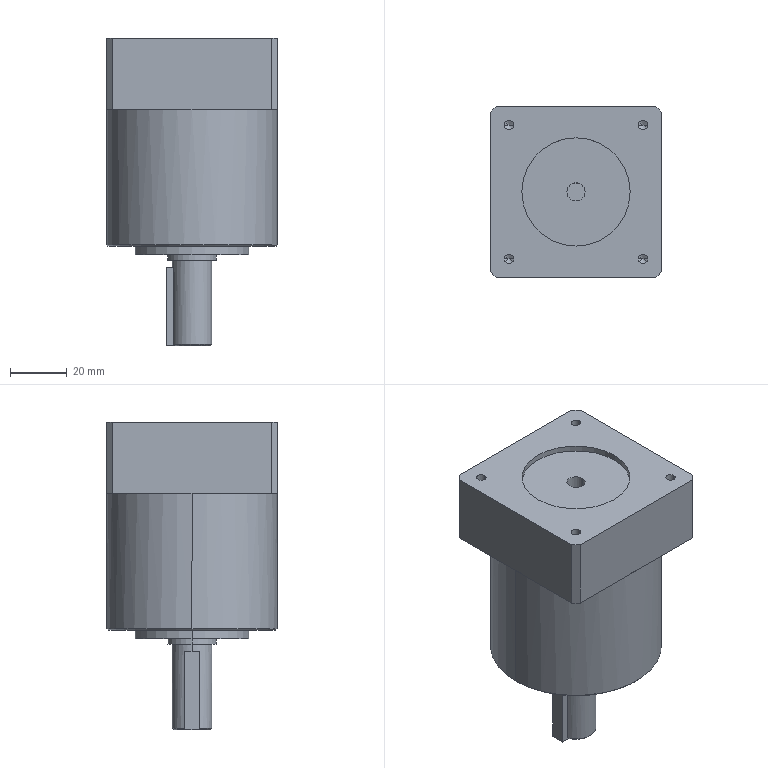Part | SolidWorks | features ICE 7, Chamfer 2, HoleWzd 2, CirPattern 1, Extrusion 1 | 1 solid | 71 faces | box 60 x 60 x 108 mm | volume 230664 mm3 | cylinder 28 | plane 23 | cone 20 | commonest cylinder face diameters 3.3 x8 4.2 x8 6.35 x2 14 x2 17 x2 38 x2